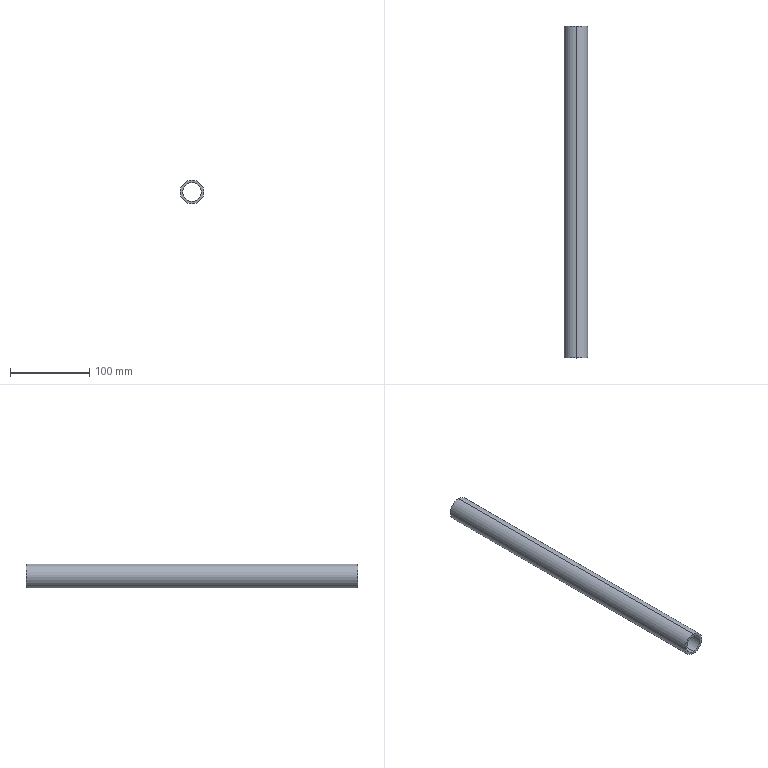Part | SolidWorks | features Extrusion 1 | 1 solid | 6 faces | box 30 x 420 x 30 mm | volume 113158 mm3 | cylinder 4 | plane 2 | commonest cylinder face diameters 23.6 x2 30 x2
STEP:
#1=CARTESIAN_POINT('',(0.,-210.,-11.8));
#2=VERTEX_POINT('',#1);
#3=CARTESIAN_POINT('',(0.,-210.,11.8));
#4=VERTEX_POINT('',#3);
#5=CARTESIAN_POINT('',(0.,-210.,0.));
#6=DIRECTION('',(0.,1.,0.));
#7=DIRECTION('',(0.,0.,1.));
#8=AXIS2_PLACEMENT_3D('',#5,#6,#7);
#9=CIRCLE('',#8,11.8);
#10=EDGE_CURVE('',#2,#4,#9,.T.);
#11=ORIENTED_EDGE('',*,*,#10,.F.);
#12=CARTESIAN_POINT('',(0.,210.,-11.8));
#13=VERTEX_POINT('',#12);
#14=CARTESIAN_POINT('',(0.,-210.,-11.8));
#15=DIRECTION('',(0.,1.,0.));
#16=VECTOR('',#15,1000.);
#17=LINE('',#14,#16);
#18=EDGE_CURVE('',#2,#13,#17,.T.);
#19=ORIENTED_EDGE('',*,*,#18,.T.);
#20=CARTESIAN_POINT('',(0.,210.,11.8));
#21=VERTEX_POINT('',#20);
#22=CARTESIAN_POINT('',(0.,210.,0.));
#23=DIRECTION('',(0.,1.,0.));
#24=DIRECTION('',(0.,0.,1.));
#25=AXIS2_PLACEMENT_3D('',#22,#23,#24);
#26=CIRCLE('',#25,11.8);
#27=EDGE_CURVE('',#13,#21,#26,.T.);
#28=ORIENTED_EDGE('',*,*,#27,.T.);
#29=CARTESIAN_POINT('',(0.,-210.,11.8));
#30=DIRECTION('',(0.,1.,0.));
#31=VECTOR('',#30,1000.);
#32=LINE('',#29,#31);
#33=EDGE_CURVE('',#4,#21,#32,.T.);
#34=ORIENTED_EDGE('',*,*,#33,.F.);
#35=EDGE_LOOP('',(#11,#19,#28,#34));
#36=FACE_OUTER_BOUND('',#35,.T.);
#37=CARTESIAN_POINT('',(0.,-210.,0.));
#38=DIRECTION('',(0.,1.,0.));
#39=DIRECTION('',(0.,0.,1.));
#40=AXIS2_PLACEMENT_3D('',#37,#38,#39);
#41=CYLINDRICAL_SURFACE('',#40,11.8);
#42=ADVANCED_FACE('',(#36),#41,.F.);
#43=CARTESIAN_POINT('',(0.,-210.,15.));
#44=VERTEX_POINT('',#43);
#45=CARTESIAN_POINT('',(0.,-210.,-15.));
#46=VERTEX_POINT('',#45);
#47=CARTESIAN_POINT('',(0.,-210.,0.));
#48=DIRECTION('',(0.,1.,0.));
#49=DIRECTION('',(0.,0.,1.));
#50=AXIS2_PLACEMENT_3D('',#47,#48,#49);
#51=CIRCLE('',#50,15.);
#52=EDGE_CURVE('',#44,#46,#51,.T.);
#53=ORIENTED_EDGE('',*,*,#52,.T.);
#54=CARTESIAN_POINT('',(0.,210.,-15.));
#55=VERTEX_POINT('',#54);
#56=CARTESIAN_POINT('',(0.,-210.,-15.));
#57=DIRECTION('',(0.,1.,0.));
#58=VECTOR('',#57,1000.);
#59=LINE('',#56,#58);
#60=EDGE_CURVE('',#46,#55,#59,.T.);
#61=ORIENTED_EDGE('',*,*,#60,.T.);
#62=CARTESIAN_POINT('',(0.,210.,15.));
#63=VERTEX_POINT('',#62);
#64=CARTESIAN_POINT('',(0.,210.,0.));
#65=DIRECTION('',(0.,1.,0.));
#66=DIRECTION('',(0.,0.,1.));
#67=AXIS2_PLACEMENT_3D('',#64,#65,#66);
#68=CIRCLE('',#67,15.);
#69=EDGE_CURVE('',#63,#55,#68,.T.);
#70=ORIENTED_EDGE('',*,*,#69,.F.);
#71=CARTESIAN_POINT('',(0.,-210.,15.));
#72=DIRECTION('',(0.,1.,0.));
#73=VECTOR('',#72,1000.);
#74=LINE('',#71,#73);
#75=EDGE_CURVE('',#44,#63,#74,.T.);
#76=ORIENTED_EDGE('',*,*,#75,.F.);
#77=EDGE_LOOP('',(#53,#61,#70,#76));
#78=FACE_OUTER_BOUND('',#77,.T.);
#79=CARTESIAN_POINT('',(0.,-210.,0.));
#80=DIRECTION('',(0.,1.,0.));
#81=DIRECTION('',(0.,0.,1.));
#82=AXIS2_PLACEMENT_3D('',#79,#80,#81);
#83=CYLINDRICAL_SURFACE('',#82,15.);
#84=ADVANCED_FACE('',(#78),#83,.T.);
#85=ORIENTED_EDGE('',*,*,#60,.F.);
#86=CARTESIAN_POINT('',(0.,-210.,0.));
#87=DIRECTION('',(0.,1.,0.));
#88=DIRECTION('',(0.,0.,1.));
#89=AXIS2_PLACEMENT_3D('',#86,#87,#88);
#90=CIRCLE('',#89,15.);
#91=EDGE_CURVE('',#46,#44,#90,.T.);
#92=ORIENTED_EDGE('',*,*,#91,.T.);
#93=ORIENTED_EDGE('',*,*,#75,.T.);
#94=CARTESIAN_POINT('',(0.,210.,0.));
#95=DIRECTION('',(0.,1.,0.));
#96=DIRECTION('',(0.,0.,1.));
#97=AXIS2_PLACEMENT_3D('',#94,#95,#96);
#98=CIRCLE('',#97,15.);
#99=EDGE_CURVE('',#55,#63,#98,.T.);
#100=ORIENTED_EDGE('',*,*,#99,.F.);
#101=EDGE_LOOP('',(#85,#92,#93,#100));
#102=FACE_OUTER_BOUND('',#101,.T.);
#103=CARTESIAN_POINT('',(0.,-210.,0.));
#104=DIRECTION('',(0.,1.,0.));
#105=DIRECTION('',(0.,0.,1.));
#106=AXIS2_PLACEMENT_3D('',#103,#104,#105);
#107=CYLINDRICAL_SURFACE('',#106,15.);
#108=ADVANCED_FACE('',(#102),#107,.T.);
#109=CARTESIAN_POINT('',(0.,-210.,0.));
#110=DIRECTION('',(0.,1.,0.));
#111=DIRECTION('',(0.,0.,1.));
#112=AXIS2_PLACEMENT_3D('',#109,#110,#111);
#113=CIRCLE('',#112,11.8);
#114=EDGE_CURVE('',#4,#2,#113,.T.);
#115=ORIENTED_EDGE('',*,*,#114,.T.);
#116=ORIENTED_EDGE('',*,*,#10,.T.);
#117=EDGE_LOOP('',(#115,#116));
#118=FACE_BOUND('',#117,.T.);
#119=ORIENTED_EDGE('',*,*,#52,.F.);
#120=ORIENTED_EDGE('',*,*,#91,.F.);
#121=EDGE_LOOP('',(#119,#120));
#122=FACE_OUTER_BOUND('',#121,.T.);
#123=CARTESIAN_POINT('',(0.,-210.,0.));
#124=DIRECTION('',(0.,1.,0.));
#125=DIRECTION('',(0.,0.,1.));
#126=AXIS2_PLACEMENT_3D('',#123,#124,#125);
#127=PLANE('',#126);
#128=ADVANCED_FACE('',(#118,#122),#127,.F.);
#129=CARTESIAN_POINT('',(0.,210.,0.));
#130=DIRECTION('',(0.,1.,0.));
#131=DIRECTION('',(0.,0.,1.));
#132=AXIS2_PLACEMENT_3D('',#129,#130,#131);
#133=CIRCLE('',#132,11.8);
#134=EDGE_CURVE('',#21,#13,#133,.T.);
#135=ORIENTED_EDGE('',*,*,#134,.F.);
#136=ORIENTED_EDGE('',*,*,#27,.F.);
#137=EDGE_LOOP('',(#135,#136));
#138=FACE_BOUND('',#137,.T.);
#139=ORIENTED_EDGE('',*,*,#69,.T.);
#140=ORIENTED_EDGE('',*,*,#99,.T.);
#141=EDGE_LOOP('',(#139,#140));
#142=FACE_OUTER_BOUND('',#141,.T.);
#143=CARTESIAN_POINT('',(0.,210.,0.));
#144=DIRECTION('',(0.,1.,0.));
#145=DIRECTION('',(0.,0.,1.));
#146=AXIS2_PLACEMENT_3D('',#143,#144,#145);
#147=PLANE('',#146);
#148=ADVANCED_FACE('',(#138,#142),#147,.T.);
#149=ORIENTED_EDGE('',*,*,#18,.F.);
#150=ORIENTED_EDGE('',*,*,#114,.F.);
#151=ORIENTED_EDGE('',*,*,#33,.T.);
#152=ORIENTED_EDGE('',*,*,#134,.T.);
#153=EDGE_LOOP('',(#149,#150,#151,#152));
#154=FACE_OUTER_BOUND('',#153,.T.);
#155=CARTESIAN_POINT('',(0.,-210.,0.));
#156=DIRECTION('',(0.,1.,0.));
#157=DIRECTION('',(0.,0.,1.));
#158=AXIS2_PLACEMENT_3D('',#155,#156,#157);
#159=CYLINDRICAL_SURFACE('',#158,11.8);
#160=ADVANCED_FACE('',(#154),#159,.F.);
#161=CLOSED_SHELL('',(#42,#84,#108,#128,#148,#160));
#162=MANIFOLD_SOLID_BREP('',#161);
#163=CARTESIAN_POINT('',(0.,0.,0.));
#164=DIRECTION('',(0.,0.,1.));
#165=DIRECTION('',(1.,0.,0.));
#166=AXIS2_PLACEMENT_3D('',#163,#164,#165);
#167=(LENGTH_UNIT()NAMED_UNIT(*)SI_UNIT(.MILLI.,.METRE.));
#168=UNCERTAINTY_MEASURE_WITH_UNIT(LENGTH_MEASURE(0.00001),#167,'','');
#169=(NAMED_UNIT(*)PLANE_ANGLE_UNIT()SI_UNIT($,.RADIAN.));
#170=(NAMED_UNIT(*)SI_UNIT($,.STERADIAN.)SOLID_ANGLE_UNIT());
#171=(GEOMETRIC_REPRESENTATION_CONTEXT(3)GLOBAL_UNCERTAINTY_ASSIGNED_CONTEXT((#168))GLOBAL_UNIT_ASSIGNED_CONTEXT((#167,#169,#170))REPRESENTATION_CONTEXT('',''));
#172=ADVANCED_BREP_SHAPE_REPRESENTATION('',(#162,#166),#171);